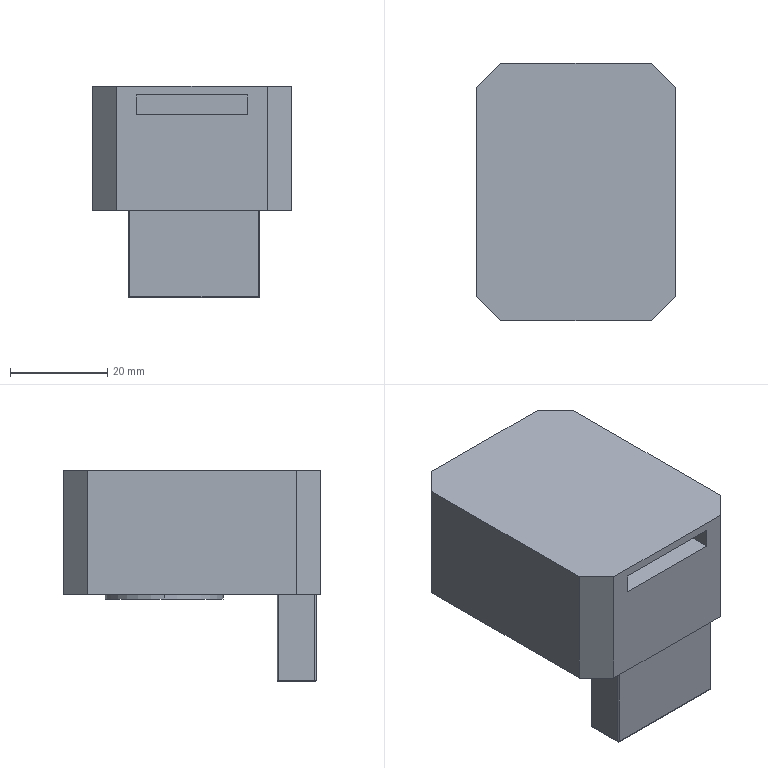Part | SolidWorks | features BaseBody 1 | 1 solid | 36 faces | box 41 x 53 x 43.5 mm | volume 58117 mm3 | plane 21 | cylinder 10 | spline 5 | commonest cylinder face diameters 0.5 x8 24.262 x2
STEP:
#1=CARTESIAN_POINT('',(6.903,-41.356,-17.75));
#2=VERTEX_POINT('',#1);
#3=CARTESIAN_POINT('',(6.977,-41.179,-17.75));
#4=VERTEX_POINT('',#3);
#5=CARTESIAN_POINT('',(6.727,-41.179,-17.75));
#6=DIRECTION('',(0.,0.,1.));
#7=DIRECTION('',(-1.,0.,0.));
#8=AXIS2_PLACEMENT_3D('',#5,#6,#7);
#9=CIRCLE('',#8,0.25);
#10=EDGE_CURVE('',#2,#4,#9,.T.);
#11=ORIENTED_EDGE('',*,*,#10,.F.);
#12=CARTESIAN_POINT('',(6.903,-41.179,-17.927));
#13=VERTEX_POINT('',#12);
#14=CARTESIAN_POINT('',(6.727,-41.179,-17.75));
#15=DIRECTION('',(0.5774,0.5774,0.5774));
#16=DIRECTION('',(-0.7071,0.,0.7071));
#17=AXIS2_PLACEMENT_3D('',#14,#15,#16);
#18=CIRCLE('',#17,0.25);
#19=EDGE_CURVE('',#2,#13,#18,.T.);
#20=ORIENTED_EDGE('',*,*,#19,.T.);
#21=CARTESIAN_POINT('',(6.727,-41.179,-17.75));
#22=DIRECTION('',(0.,1.,0.));
#23=DIRECTION('',(-1.,0.,0.));
#24=AXIS2_PLACEMENT_3D('',#21,#22,#23);
#25=CIRCLE('',#24,0.25);
#26=EDGE_CURVE('',#4,#13,#25,.T.);
#27=ORIENTED_EDGE('',*,*,#26,.F.);
#28=EDGE_LOOP('',(#11,#20,#27));
#29=FACE_OUTER_BOUND('',#28,.T.);
#30=CARTESIAN_POINT('',(6.903,-41.357,-17.749));
#31=CARTESIAN_POINT('',(6.944,-41.315,-17.707));
#32=CARTESIAN_POINT('',(6.968,-41.251,-17.684));
#33=CARTESIAN_POINT('',(6.968,-41.179,-17.684));
#34=CARTESIAN_POINT('',(6.941,-41.32,-17.824));
#35=CARTESIAN_POINT('',(6.974,-41.287,-17.791));
#36=CARTESIAN_POINT('',(6.992,-41.236,-17.773));
#37=CARTESIAN_POINT('',(6.992,-41.179,-17.773));
#38=CARTESIAN_POINT('',(6.941,-41.255,-17.889));
#39=CARTESIAN_POINT('',(6.959,-41.237,-17.872));
#40=CARTESIAN_POINT('',(6.969,-41.21,-17.862));
#41=CARTESIAN_POINT('',(6.969,-41.179,-17.862));
#42=CARTESIAN_POINT('',(6.903,-41.179,-17.927));
#43=CARTESIAN_POINT('',(6.903,-41.179,-17.927));
#44=CARTESIAN_POINT('',(6.903,-41.179,-17.927));
#45=CARTESIAN_POINT('',(6.903,-41.179,-17.927));
#46=(BOUNDED_SURFACE()B_SPLINE_SURFACE(3,3,((#30,#31,#32,#33),(#34,#35,#36,#37),(#38,#39,#40,#41),(#42,#43,#44,#45)),.UNSPECIFIED.,.F.,.F.,.F.)B_SPLINE_SURFACE_WITH_KNOTS((4,4),(4,4),(0.,1.),(0.,1.),.UNSPECIFIED.)GEOMETRIC_REPRESENTATION_ITEM()RATIONAL_B_SPLINE_SURFACE(((1.,0.9254,0.9254,1.),(0.9096,0.8418,0.8418,0.9096),(0.9096,0.8418,0.8418,0.9096),(1.,0.9254,0.9254,1.)))REPRESENTATION_ITEM('')SURFACE());
#47=ADVANCED_FACE('',(#29),#46,.T.);
#48=CARTESIAN_POINT('',(-19.304,-10.179,0.));
#49=VERTEX_POINT('',#48);
#50=CARTESIAN_POINT('',(4.957,-10.179,0.));
#51=VERTEX_POINT('',#50);
#52=CARTESIAN_POINT('',(-7.173,-10.179,0.));
#53=DIRECTION('',(0.,0.,-1.));
#54=DIRECTION('',(-1.,0.,0.));
#55=AXIS2_PLACEMENT_3D('',#52,#53,#54);
#56=CIRCLE('',#55,12.131);
#57=EDGE_CURVE('',#49,#51,#56,.T.);
#58=ORIENTED_EDGE('',*,*,#57,.T.);
#59=CARTESIAN_POINT('',(4.957,-10.179,-1.));
#60=VERTEX_POINT('',#59);
#61=CARTESIAN_POINT('',(4.957,-10.179,0.));
#62=DIRECTION('',(0.,0.,-1.));
#63=VECTOR('',#62,1000.);
#64=LINE('',#61,#63);
#65=EDGE_CURVE('',#51,#60,#64,.T.);
#66=ORIENTED_EDGE('',*,*,#65,.T.);
#67=CARTESIAN_POINT('',(-19.304,-10.179,-1.));
#68=VERTEX_POINT('',#67);
#69=CARTESIAN_POINT('',(-7.173,-10.179,-1.));
#70=DIRECTION('',(0.,0.,1.));
#71=DIRECTION('',(-1.,0.,0.));
#72=AXIS2_PLACEMENT_3D('',#69,#70,#71);
#73=CIRCLE('',#72,12.131);
#74=EDGE_CURVE('',#60,#68,#73,.T.);
#75=ORIENTED_EDGE('',*,*,#74,.T.);
#76=CARTESIAN_POINT('',(-19.304,-10.179,0.));
#77=DIRECTION('',(0.,0.,-1.));
#78=VECTOR('',#77,1000.);
#79=LINE('',#76,#78);
#80=EDGE_CURVE('',#49,#68,#79,.T.);
#81=ORIENTED_EDGE('',*,*,#80,.F.);
#82=EDGE_LOOP('',(#58,#66,#75,#81));
#83=FACE_OUTER_BOUND('',#82,.T.);
#84=CARTESIAN_POINT('',(-7.173,-10.179,0.));
#85=DIRECTION('',(0.,0.,-1.));
#86=DIRECTION('',(-1.,0.,0.));
#87=AXIS2_PLACEMENT_3D('',#84,#85,#86);
#88=CYLINDRICAL_SURFACE('',#87,12.131);
#89=ADVANCED_FACE('',(#83),#88,.T.);
#90=CARTESIAN_POINT('',(-22.423,10.571,25.5));
#91=VERTEX_POINT('',#90);
#92=CARTESIAN_POINT('',(-27.423,5.571,25.5));
#93=VERTEX_POINT('',#92);
#94=CARTESIAN_POINT('',(-22.423,10.571,25.5));
#95=DIRECTION('',(-0.7071,-0.7071,0.));
#96=VECTOR('',#95,1000.);
#97=LINE('',#94,#96);
#98=EDGE_CURVE('',#91,#93,#97,.T.);
#99=ORIENTED_EDGE('',*,*,#98,.T.);
#100=CARTESIAN_POINT('',(-27.423,-37.429,25.5));
#101=VERTEX_POINT('',#100);
#102=CARTESIAN_POINT('',(-27.423,-15.929,25.5));
#103=DIRECTION('',(0.,-1.,0.));
#104=VECTOR('',#103,1000.);
#105=LINE('',#102,#104);
#106=EDGE_CURVE('',#93,#101,#105,.T.);
#107=ORIENTED_EDGE('',*,*,#106,.T.);
#108=CARTESIAN_POINT('',(-22.423,-42.429,25.5));
#109=VERTEX_POINT('',#108);
#110=CARTESIAN_POINT('',(-27.423,-37.429,25.5));
#111=DIRECTION('',(0.7071,-0.7071,0.));
#112=VECTOR('',#111,1000.);
#113=LINE('',#110,#112);
#114=EDGE_CURVE('',#101,#109,#113,.T.);
#115=ORIENTED_EDGE('',*,*,#114,.T.);
#116=CARTESIAN_POINT('',(8.577,-42.429,25.5));
#117=VERTEX_POINT('',#116);
#118=CARTESIAN_POINT('',(-6.923,-42.429,25.5));
#119=DIRECTION('',(1.,0.,0.));
#120=VECTOR('',#119,1000.);
#121=LINE('',#118,#120);
#122=EDGE_CURVE('',#109,#117,#121,.T.);
#123=ORIENTED_EDGE('',*,*,#122,.T.);
#124=CARTESIAN_POINT('',(13.577,-37.429,25.5));
#125=VERTEX_POINT('',#124);
#126=CARTESIAN_POINT('',(8.577,-42.429,25.5));
#127=DIRECTION('',(0.7071,0.7071,0.));
#128=VECTOR('',#127,1000.);
#129=LINE('',#126,#128);
#130=EDGE_CURVE('',#117,#125,#129,.T.);
#131=ORIENTED_EDGE('',*,*,#130,.T.);
#132=CARTESIAN_POINT('',(13.577,5.571,25.5));
#133=VERTEX_POINT('',#132);
#134=CARTESIAN_POINT('',(13.577,-15.929,25.5));
#135=DIRECTION('',(0.,1.,0.));
#136=VECTOR('',#135,1000.);
#137=LINE('',#134,#136);
#138=EDGE_CURVE('',#125,#133,#137,.T.);
#139=ORIENTED_EDGE('',*,*,#138,.T.);
#140=CARTESIAN_POINT('',(8.577,10.571,25.5));
#141=VERTEX_POINT('',#140);
#142=CARTESIAN_POINT('',(13.577,5.571,25.5));
#143=DIRECTION('',(-0.7071,0.7071,0.));
#144=VECTOR('',#143,1000.);
#145=LINE('',#142,#144);
#146=EDGE_CURVE('',#133,#141,#145,.T.);
#147=ORIENTED_EDGE('',*,*,#146,.T.);
#148=CARTESIAN_POINT('',(-6.923,10.571,25.5));
#149=DIRECTION('',(-1.,0.,0.));
#150=VECTOR('',#149,1000.);
#151=LINE('',#148,#150);
#152=EDGE_CURVE('',#141,#91,#151,.T.);
#153=ORIENTED_EDGE('',*,*,#152,.T.);
#154=EDGE_LOOP('',(#99,#107,#115,#123,#131,#139,#147,#153));
#155=FACE_OUTER_BOUND('',#154,.T.);
#156=CARTESIAN_POINT('',(-6.923,-15.929,25.5));
#157=DIRECTION('',(0.,0.,1.));
#158=DIRECTION('',(1.,0.,0.));
#159=AXIS2_PLACEMENT_3D('',#156,#157,#158);
#160=PLANE('',#159);
#161=ADVANCED_FACE('',(#155),#160,.T.);
#162=CARTESIAN_POINT('',(-27.423,5.571,0.));
#163=VERTEX_POINT('',#162);
#164=CARTESIAN_POINT('',(-27.423,5.571,0.));
#165=DIRECTION('',(0.,0.,-1.));
#166=VECTOR('',#165,1000.);
#167=LINE('',#164,#166);
#168=EDGE_CURVE('',#93,#163,#167,.T.);
#169=ORIENTED_EDGE('',*,*,#168,.T.);
#170=CARTESIAN_POINT('',(-27.423,-37.429,0.));
#171=VERTEX_POINT('',#170);
#172=CARTESIAN_POINT('',(-27.423,-42.429,0.));
#173=DIRECTION('',(0.,-1.,0.));
#174=VECTOR('',#173,1000.);
#175=LINE('',#172,#174);
#176=EDGE_CURVE('',#163,#171,#175,.T.);
#177=ORIENTED_EDGE('',*,*,#176,.T.);
#178=CARTESIAN_POINT('',(-27.423,-37.429,0.));
#179=DIRECTION('',(0.,0.,1.));
#180=VECTOR('',#179,1000.);
#181=LINE('',#178,#180);
#182=EDGE_CURVE('',#171,#101,#181,.T.);
#183=ORIENTED_EDGE('',*,*,#182,.T.);
#184=ORIENTED_EDGE('',*,*,#106,.F.);
#185=EDGE_LOOP('',(#169,#177,#183,#184));
#186=FACE_OUTER_BOUND('',#185,.T.);
#187=CARTESIAN_POINT('',(-27.423,-42.429,0.));
#188=DIRECTION('',(-1.,0.,0.));
#189=DIRECTION('',(0.,0.,1.));
#190=AXIS2_PLACEMENT_3D('',#187,#188,#189);
#191=PLANE('',#190);
#192=ADVANCED_FACE('',(#186),#191,.T.);
#193=CARTESIAN_POINT('',(-22.423,10.571,0.));
#194=VERTEX_POINT('',#193);
#195=CARTESIAN_POINT('',(-24.923,8.071,0.));
#196=DIRECTION('',(-0.7071,-0.7071,0.));
#197=VECTOR('',#196,1000.);
#198=LINE('',#195,#197);
#199=EDGE_CURVE('',#194,#163,#198,.T.);
#200=ORIENTED_EDGE('',*,*,#199,.T.);
#201=ORIENTED_EDGE('',*,*,#168,.F.);
#202=ORIENTED_EDGE('',*,*,#98,.F.);
#203=CARTESIAN_POINT('',(-22.423,10.571,0.));
#204=DIRECTION('',(0.,0.,-1.));
#205=VECTOR('',#204,1000.);
#206=LINE('',#203,#205);
#207=EDGE_CURVE('',#91,#194,#206,.T.);
#208=ORIENTED_EDGE('',*,*,#207,.T.);
#209=EDGE_LOOP('',(#200,#201,#202,#208));
#210=FACE_OUTER_BOUND('',#209,.T.);
#211=CARTESIAN_POINT('',(-24.923,8.071,0.));
#212=DIRECTION('',(-0.7071,0.7071,0.));
#213=DIRECTION('',(-0.7071,-0.7071,0.));
#214=AXIS2_PLACEMENT_3D('',#211,#212,#213);
#215=PLANE('',#214);
#216=ADVANCED_FACE('',(#210),#215,.T.);
#217=ORIENTED_EDGE('',*,*,#207,.F.);
#218=ORIENTED_EDGE('',*,*,#152,.F.);
#219=CARTESIAN_POINT('',(8.577,10.571,0.));
#220=VERTEX_POINT('',#219);
#221=CARTESIAN_POINT('',(8.577,10.571,0.));
#222=DIRECTION('',(0.,0.,-1.));
#223=VECTOR('',#222,1000.);
#224=LINE('',#221,#223);
#225=EDGE_CURVE('',#141,#220,#224,.T.);
#226=ORIENTED_EDGE('',*,*,#225,.T.);
#227=CARTESIAN_POINT('',(-27.423,10.571,0.));
#228=DIRECTION('',(-1.,0.,0.));
#229=VECTOR('',#228,1000.);
#230=LINE('',#227,#229);
#231=EDGE_CURVE('',#220,#194,#230,.T.);
#232=ORIENTED_EDGE('',*,*,#231,.T.);
#233=EDGE_LOOP('',(#217,#218,#226,#232));
#234=FACE_OUTER_BOUND('',#233,.T.);
#235=CARTESIAN_POINT('',(-27.423,10.571,0.));
#236=DIRECTION('',(0.,1.,0.));
#237=DIRECTION('',(0.,0.,1.));
#238=AXIS2_PLACEMENT_3D('',#235,#236,#237);
#239=PLANE('',#238);
#240=ADVANCED_FACE('',(#234),#239,.T.);
#241=CARTESIAN_POINT('',(13.577,5.571,0.));
#242=VERTEX_POINT('',#241);
#243=CARTESIAN_POINT('',(11.077,8.071,0.));
#244=DIRECTION('',(-0.7071,0.7071,0.));
#245=VECTOR('',#244,1000.);
#246=LINE('',#243,#245);
#247=EDGE_CURVE('',#242,#220,#246,.T.);
#248=ORIENTED_EDGE('',*,*,#247,.T.);
#249=ORIENTED_EDGE('',*,*,#225,.F.);
#250=ORIENTED_EDGE('',*,*,#146,.F.);
#251=CARTESIAN_POINT('',(13.577,5.571,0.));
#252=DIRECTION('',(0.,0.,-1.));
#253=VECTOR('',#252,1000.);
#254=LINE('',#251,#253);
#255=EDGE_CURVE('',#133,#242,#254,.T.);
#256=ORIENTED_EDGE('',*,*,#255,.T.);
#257=EDGE_LOOP('',(#248,#249,#250,#256));
#258=FACE_OUTER_BOUND('',#257,.T.);
#259=CARTESIAN_POINT('',(11.077,8.071,0.));
#260=DIRECTION('',(0.7071,0.7071,0.));
#261=DIRECTION('',(-0.7071,0.7071,0.));
#262=AXIS2_PLACEMENT_3D('',#259,#260,#261);
#263=PLANE('',#262);
#264=ADVANCED_FACE('',(#258),#263,.T.);
#265=ORIENTED_EDGE('',*,*,#255,.F.);
#266=ORIENTED_EDGE('',*,*,#138,.F.);
#267=CARTESIAN_POINT('',(13.577,-37.429,0.));
#268=VERTEX_POINT('',#267);
#269=CARTESIAN_POINT('',(13.577,-37.429,0.));
#270=DIRECTION('',(0.,0.,-1.));
#271=VECTOR('',#270,1000.);
#272=LINE('',#269,#271);
#273=EDGE_CURVE('',#125,#268,#272,.T.);
#274=ORIENTED_EDGE('',*,*,#273,.T.);
#275=CARTESIAN_POINT('',(13.577,10.571,0.));
#276=DIRECTION('',(0.,1.,0.));
#277=VECTOR('',#276,1000.);
#278=LINE('',#275,#277);
#279=EDGE_CURVE('',#268,#242,#278,.T.);
#280=ORIENTED_EDGE('',*,*,#279,.T.);
#281=EDGE_LOOP('',(#265,#266,#274,#280));
#282=FACE_OUTER_BOUND('',#281,.T.);
#283=CARTESIAN_POINT('',(13.577,10.571,0.));
#284=DIRECTION('',(1.,0.,0.));
#285=DIRECTION('',(0.,0.,-1.));
#286=AXIS2_PLACEMENT_3D('',#283,#284,#285);
#287=PLANE('',#286);
#288=ADVANCED_FACE('',(#282),#287,.T.);
#289=CARTESIAN_POINT('',(8.577,-42.429,0.));
#290=VERTEX_POINT('',#289);
#291=CARTESIAN_POINT('',(11.077,-39.929,0.));
#292=DIRECTION('',(0.7071,0.7071,0.));
#293=VECTOR('',#292,1000.);
#294=LINE('',#291,#293);
#295=EDGE_CURVE('',#290,#268,#294,.T.);
#296=ORIENTED_EDGE('',*,*,#295,.T.);
#297=ORIENTED_EDGE('',*,*,#273,.F.);
#298=ORIENTED_EDGE('',*,*,#130,.F.);
#299=CARTESIAN_POINT('',(8.577,-42.429,0.));
#300=DIRECTION('',(0.,0.,-1.));
#301=VECTOR('',#300,1000.);
#302=LINE('',#299,#301);
#303=EDGE_CURVE('',#117,#290,#302,.T.);
#304=ORIENTED_EDGE('',*,*,#303,.T.);
#305=EDGE_LOOP('',(#296,#297,#298,#304));
#306=FACE_OUTER_BOUND('',#305,.T.);
#307=CARTESIAN_POINT('',(11.077,-39.929,0.));
#308=DIRECTION('',(0.7071,-0.7071,0.));
#309=DIRECTION('',(0.7071,0.7071,0.));
#310=AXIS2_PLACEMENT_3D('',#307,#308,#309);
#311=PLANE('',#310);
#312=ADVANCED_FACE('',(#306),#311,.T.);
#313=CARTESIAN_POINT('',(-18.423,-42.429,19.7));
#314=VERTEX_POINT('',#313);
#315=CARTESIAN_POINT('',(-18.423,-42.429,23.7));
#316=VERTEX_POINT('',#315);
#317=CARTESIAN_POINT('',(-18.423,-42.429,0.));
#318=DIRECTION('',(0.,0.,1.));
#319=VECTOR('',#318,1000.);
#320=LINE('',#317,#319);
#321=EDGE_CURVE('',#314,#316,#320,.T.);
#322=ORIENTED_EDGE('',*,*,#321,.T.);
#323=CARTESIAN_POINT('',(4.577,-42.429,23.7));
#324=VERTEX_POINT('',#323);
#325=CARTESIAN_POINT('',(13.577,-42.429,23.7));
#326=DIRECTION('',(1.,0.,0.));
#327=VECTOR('',#326,1000.);
#328=LINE('',#325,#327);
#329=EDGE_CURVE('',#316,#324,#328,.T.);
#330=ORIENTED_EDGE('',*,*,#329,.T.);
#331=CARTESIAN_POINT('',(4.577,-42.429,19.7));
#332=VERTEX_POINT('',#331);
#333=CARTESIAN_POINT('',(4.577,-42.429,0.));
#334=DIRECTION('',(0.,0.,-1.));
#335=VECTOR('',#334,1000.);
#336=LINE('',#333,#335);
#337=EDGE_CURVE('',#324,#332,#336,.T.);
#338=ORIENTED_EDGE('',*,*,#337,.T.);
#339=CARTESIAN_POINT('',(13.577,-42.429,19.7));
#340=DIRECTION('',(-1.,0.,0.));
#341=VECTOR('',#340,1000.);
#342=LINE('',#339,#341);
#343=EDGE_CURVE('',#332,#314,#342,.T.);
#344=ORIENTED_EDGE('',*,*,#343,.T.);
#345=EDGE_LOOP('',(#322,#330,#338,#344));
#346=FACE_BOUND('',#345,.T.);
#347=ORIENTED_EDGE('',*,*,#303,.F.);
#348=ORIENTED_EDGE('',*,*,#122,.F.);
#349=CARTESIAN_POINT('',(-22.423,-42.429,0.));
#350=VERTEX_POINT('',#349);
#351=CARTESIAN_POINT('',(-22.423,-42.429,0.));
#352=DIRECTION('',(0.,0.,-1.));
#353=VECTOR('',#352,1000.);
#354=LINE('',#351,#353);
#355=EDGE_CURVE('',#109,#350,#354,.T.);
#356=ORIENTED_EDGE('',*,*,#355,.T.);
#357=CARTESIAN_POINT('',(13.577,-42.429,0.));
#358=DIRECTION('',(1.,0.,0.));
#359=VECTOR('',#358,1000.);
#360=LINE('',#357,#359);
#361=EDGE_CURVE('',#350,#290,#360,.T.);
#362=ORIENTED_EDGE('',*,*,#361,.T.);
#363=EDGE_LOOP('',(#347,#348,#356,#362));
#364=FACE_OUTER_BOUND('',#363,.T.);
#365=CARTESIAN_POINT('',(13.577,-42.429,0.));
#366=DIRECTION('',(0.,-1.,0.));
#367=DIRECTION('',(0.,0.,-1.));
#368=AXIS2_PLACEMENT_3D('',#365,#366,#367);
#369=PLANE('',#368);
#370=ADVANCED_FACE('',(#346,#364),#369,.T.);
#371=CARTESIAN_POINT('',(-24.923,-39.929,0.));
#372=DIRECTION('',(0.7071,-0.7071,0.));
#373=VECTOR('',#372,1000.);
#374=LINE('',#371,#373);
#375=EDGE_CURVE('',#171,#350,#374,.T.);
#376=ORIENTED_EDGE('',*,*,#375,.T.);
#377=ORIENTED_EDGE('',*,*,#355,.F.);
#378=ORIENTED_EDGE('',*,*,#114,.F.);
#379=ORIENTED_EDGE('',*,*,#182,.F.);
#380=EDGE_LOOP('',(#376,#377,#378,#379));
#381=FACE_OUTER_BOUND('',#380,.T.);
#382=CARTESIAN_POINT('',(-24.923,-39.929,0.));
#383=DIRECTION('',(-0.7071,-0.7071,0.));
#384=DIRECTION('',(0.7071,-0.7071,0.));
#385=AXIS2_PLACEMENT_3D('',#382,#383,#384);
#386=PLANE('',#385);
#387=ADVANCED_FACE('',(#381),#386,.T.);
#388=CARTESIAN_POINT('',(-19.773,-41.429,0.));
#389=VERTEX_POINT('',#388);
#390=CARTESIAN_POINT('',(-20.023,-41.179,0.));
#391=VERTEX_POINT('',#390);
#392=CARTESIAN_POINT('',(-19.773,-41.179,0.));
#393=DIRECTION('',(0.,0.,-1.));
#394=DIRECTION('',(-1.,0.,0.));
#395=AXIS2_PLACEMENT_3D('',#392,#393,#394);
#396=CIRCLE('',#395,0.25);
#397=EDGE_CURVE('',#389,#391,#396,.T.);
#398=ORIENTED_EDGE('',*,*,#397,.F.);
#399=CARTESIAN_POINT('',(6.727,-41.429,0.));
#400=VERTEX_POINT('',#399);
#401=CARTESIAN_POINT('',(-6.923,-41.429,0.));
#402=DIRECTION('',(-1.,0.,0.));
#403=VECTOR('',#402,1000.);
#404=LINE('',#401,#403);
#405=EDGE_CURVE('',#400,#389,#404,.T.);
#406=ORIENTED_EDGE('',*,*,#405,.F.);
#407=CARTESIAN_POINT('',(6.977,-41.179,0.));
#408=VERTEX_POINT('',#407);
#409=CARTESIAN_POINT('',(6.727,-41.179,0.));
#410=DIRECTION('',(0.,0.,-1.));
#411=DIRECTION('',(-1.,0.,0.));
#412=AXIS2_PLACEMENT_3D('',#409,#410,#411);
#413=CIRCLE('',#412,0.25);
#414=EDGE_CURVE('',#408,#400,#413,.T.);
#415=ORIENTED_EDGE('',*,*,#414,.F.);
#416=CARTESIAN_POINT('',(6.977,-33.679,0.));
#417=VERTEX_POINT('',#416);
#418=CARTESIAN_POINT('',(6.977,-15.929,0.));
#419=DIRECTION('',(0.,-1.,0.));
#420=VECTOR('',#419,1000.);
#421=LINE('',#418,#420);
#422=EDGE_CURVE('',#417,#408,#421,.T.);
#423=ORIENTED_EDGE('',*,*,#422,.F.);
#424=CARTESIAN_POINT('',(6.727,-33.429,0.));
#425=VERTEX_POINT('',#424);
#426=CARTESIAN_POINT('',(6.727,-33.679,0.));
#427=DIRECTION('',(0.,0.,-1.));
#428=DIRECTION('',(-1.,0.,0.));
#429=AXIS2_PLACEMENT_3D('',#426,#427,#428);
#430=CIRCLE('',#429,0.25);
#431=EDGE_CURVE('',#425,#417,#430,.T.);
#432=ORIENTED_EDGE('',*,*,#431,.F.);
#433=CARTESIAN_POINT('',(-19.773,-33.429,0.));
#434=VERTEX_POINT('',#433);
#435=CARTESIAN_POINT('',(-6.923,-33.429,0.));
#436=DIRECTION('',(1.,0.,0.));
#437=VECTOR('',#436,1000.);
#438=LINE('',#435,#437);
#439=EDGE_CURVE('',#434,#425,#438,.T.);
#440=ORIENTED_EDGE('',*,*,#439,.F.);
#441=CARTESIAN_POINT('',(-20.023,-33.679,0.));
#442=VERTEX_POINT('',#441);
#443=CARTESIAN_POINT('',(-19.773,-33.679,0.));
#444=DIRECTION('',(0.,0.,-1.));
#445=DIRECTION('',(-1.,0.,0.));
#446=AXIS2_PLACEMENT_3D('',#443,#444,#445);
#447=CIRCLE('',#446,0.25);
#448=EDGE_CURVE('',#442,#434,#447,.T.);
#449=ORIENTED_EDGE('',*,*,#448,.F.);
#450=CARTESIAN_POINT('',(-20.023,-15.929,0.));
#451=DIRECTION('',(0.,1.,0.));
#452=VECTOR('',#451,1000.);
#453=LINE('',#450,#452);
#454=EDGE_CURVE('',#391,#442,#453,.T.);
#455=ORIENTED_EDGE('',*,*,#454,.F.);
#456=EDGE_LOOP('',(#398,#406,#415,#423,#432,#440,#449,#455));
#457=FACE_BOUND('',#456,.T.);
#458=ORIENTED_EDGE('',*,*,#57,.F.);
#459=CARTESIAN_POINT('',(-7.173,-10.179,0.));
#460=DIRECTION('',(0.,0.,-1.));
#461=DIRECTION('',(-1.,0.,0.));
#462=AXIS2_PLACEMENT_3D('',#459,#460,#461);
#463=CIRCLE('',#462,12.131);
#464=EDGE_CURVE('',#51,#49,#463,.T.);
#465=ORIENTED_EDGE('',*,*,#464,.F.);
#466=EDGE_LOOP('',(#458,#465));
#467=FACE_BOUND('',#466,.T.);
#468=ORIENTED_EDGE('',*,*,#176,.F.);
#469=ORIENTED_EDGE('',*,*,#199,.F.);
#470=ORIENTED_EDGE('',*,*,#231,.F.);
#471=ORIENTED_EDGE('',*,*,#247,.F.);
#472=ORIENTED_EDGE('',*,*,#279,.F.);
#473=ORIENTED_EDGE('',*,*,#295,.F.);
#474=ORIENTED_EDGE('',*,*,#361,.F.);
#475=ORIENTED_EDGE('',*,*,#375,.F.);
#476=EDGE_LOOP('',(#468,#469,#470,#471,#472,#473,#474,#475));
#477=FACE_OUTER_BOUND('',#476,.T.);
#478=CARTESIAN_POINT('',(-6.923,-15.929,0.));
#479=DIRECTION('',(0.,0.,1.));
#480=DIRECTION('',(1.,0.,0.));
#481=AXIS2_PLACEMENT_3D('',#478,#479,#480);
#482=PLANE('',#481);
#483=ADVANCED_FACE('',(#457,#467,#477),#482,.F.);
#484=CARTESIAN_POINT('',(4.577,-38.429,23.7));
#485=VERTEX_POINT('',#484);
#486=CARTESIAN_POINT('',(4.577,-42.429,23.7));
#487=DIRECTION('',(0.,1.,0.));
#488=VECTOR('',#487,1000.);
#489=LINE('',#486,#488);
#490=EDGE_CURVE('',#324,#485,#489,.T.);
#491=ORIENTED_EDGE('',*,*,#490,.F.);
#492=ORIENTED_EDGE('',*,*,#329,.F.);
#493=CARTESIAN_POINT('',(-18.423,-38.429,23.7));
#494=VERTEX_POINT('',#493);
#495=CARTESIAN_POINT('',(-18.423,-42.429,23.7));
#496=DIRECTION('',(0.,-1.,0.));
#497=VECTOR('',#496,1000.);
#498=LINE('',#495,#497);
#499=EDGE_CURVE('',#494,#316,#498,.T.);
#500=ORIENTED_EDGE('',*,*,#499,.F.);
#501=CARTESIAN_POINT('',(4.577,-38.429,23.7));
#502=DIRECTION('',(-1.,0.,0.));
#503=VECTOR('',#502,1000.);
#504=LINE('',#501,#503);
#505=EDGE_CURVE('',#485,#494,#504,.T.);
#506=ORIENTED_EDGE('',*,*,#505,.F.);
#507=EDGE_LOOP('',(#491,#492,#500,#506));
#508=FACE_OUTER_BOUND('',#507,.T.);
#509=CARTESIAN_POINT('',(4.577,-42.429,23.7));
#510=DIRECTION('',(0.,0.,1.));
#511=DIRECTION('',(1.,0.,0.));
#512=AXIS2_PLACEMENT_3D('',#509,#510,#511);
#513=PLANE('',#512);
#514=ADVANCED_FACE('',(#508),#513,.F.);
#515=ORIENTED_EDGE('',*,*,#499,.T.);
#516=ORIENTED_EDGE('',*,*,#321,.F.);
#517=CARTESIAN_POINT('',(-18.423,-38.429,19.7));
#518=VERTEX_POINT('',#517);
#519=CARTESIAN_POINT('',(-18.423,-42.429,19.7));
#520=DIRECTION('',(0.,-1.,0.));
#521=VECTOR('',#520,1000.);
#522=LINE('',#519,#521);
#523=EDGE_CURVE('',#518,#314,#522,.T.);
#524=ORIENTED_EDGE('',*,*,#523,.F.);
#525=CARTESIAN_POINT('',(-18.423,-38.429,23.7));
#526=DIRECTION('',(0.,0.,-1.));
#527=VECTOR('',#526,1000.);
#528=LINE('',#525,#527);
#529=EDGE_CURVE('',#494,#518,#528,.T.);
#530=ORIENTED_EDGE('',*,*,#529,.F.);
#531=EDGE_LOOP('',(#515,#516,#524,#530));
#532=FACE_OUTER_BOUND('',#531,.T.);
#533=CARTESIAN_POINT('',(-18.423,-42.429,23.7));
#534=DIRECTION('',(-1.,0.,0.));
#535=DIRECTION('',(0.,0.,1.));
#536=AXIS2_PLACEMENT_3D('',#533,#534,#535);
#537=PLANE('',#536);
#538=ADVANCED_FACE('',(#532),#537,.F.);
#539=ORIENTED_EDGE('',*,*,#523,.T.);
#540=ORIENTED_EDGE('',*,*,#343,.F.);
#541=CARTESIAN_POINT('',(4.577,-38.429,19.7));
#542=VERTEX_POINT('',#541);
#543=CARTESIAN_POINT('',(4.577,-42.429,19.7));
#544=DIRECTION('',(0.,-1.,0.));
#545=VECTOR('',#544,1000.);
#546=LINE('',#543,#545);
#547=EDGE_CURVE('',#542,#332,#546,.T.);
#548=ORIENTED_EDGE('',*,*,#547,.F.);
#549=CARTESIAN_POINT('',(-18.423,-38.429,19.7));
#550=DIRECTION('',(1.,0.,0.));
#551=VECTOR('',#550,1000.);
#552=LINE('',#549,#551);
#553=EDGE_CURVE('',#518,#542,#552,.T.);
#554=ORIENTED_EDGE('',*,*,#553,.F.);
#555=EDGE_LOOP('',(#539,#540,#548,#554));
#556=FACE_OUTER_BOUND('',#555,.T.);
#557=CARTESIAN_POINT('',(-18.423,-42.429,19.7));
#558=DIRECTION('',(0.,0.,-1.));
#559=DIRECTION('',(-1.,0.,0.));
#560=AXIS2_PLACEMENT_3D('',#557,#558,#559);
#561=PLANE('',#560);
#562=ADVANCED_FACE('',(#556),#561,.F.);
#563=ORIENTED_EDGE('',*,*,#547,.T.);
#564=ORIENTED_EDGE('',*,*,#337,.F.);
#565=ORIENTED_EDGE('',*,*,#490,.T.);
#566=CARTESIAN_POINT('',(4.577,-38.429,19.7));
#567=DIRECTION('',(0.,0.,1.));
#568=VECTOR('',#567,1000.);
#569=LINE('',#566,#568);
#570=EDGE_CURVE('',#542,#485,#569,.T.);
#571=ORIENTED_EDGE('',*,*,#570,.F.);
#572=EDGE_LOOP('',(#563,#564,#565,#571));
#573=FACE_OUTER_BOUND('',#572,.T.);
#574=CARTESIAN_POINT('',(4.577,-42.429,19.7));
#575=DIRECTION('',(1.,0.,0.));
#576=DIRECTION('',(0.,0.,-1.));
#577=AXIS2_PLACEMENT_3D('',#574,#575,#576);
#578=PLANE('',#577);
#579=ADVANCED_FACE('',(#573),#578,.F.);
#580=CARTESIAN_POINT('',(-20.023,-41.179,-17.75));
#581=VERTEX_POINT('',#580);
#582=CARTESIAN_POINT('',(-20.023,-41.179,0.));
#583=DIRECTION('',(0.,0.,1.));
#584=VECTOR('',#583,1000.);
#585=LINE('',#582,#584);
#586=EDGE_CURVE('',#581,#391,#585,.T.);
#587=ORIENTED_EDGE('',*,*,#586,.T.);
#588=ORIENTED_EDGE('',*,*,#454,.T.);
#589=CARTESIAN_POINT('',(-20.023,-33.679,-17.75));
#590=VERTEX_POINT('',#589);
#591=CARTESIAN_POINT('',(-20.023,-33.679,0.));
#592=DIRECTION('',(0.,0.,-1.));
#593=VECTOR('',#592,1000.);
#594=LINE('',#591,#593);
#595=EDGE_CURVE('',#442,#590,#594,.T.);
#596=ORIENTED_EDGE('',*,*,#595,.T.);
#597=CARTESIAN_POINT('',(-20.023,-33.429,-17.75));
#598=DIRECTION('',(0.,-1.,0.));
#599=VECTOR('',#598,1000.);
#600=LINE('',#597,#599);
#601=EDGE_CURVE('',#590,#581,#600,.T.);
#602=ORIENTED_EDGE('',*,*,#601,.T.);
#603=EDGE_LOOP('',(#587,#588,#596,#602));
#604=FACE_OUTER_BOUND('',#603,.T.);
#605=CARTESIAN_POINT('',(-20.023,-33.429,0.));
#606=DIRECTION('',(-1.,0.,0.));
#607=DIRECTION('',(0.,0.,1.));
#608=AXIS2_PLACEMENT_3D('',#605,#606,#607);
#609=PLANE('',#608);
#610=ADVANCED_FACE('',(#604),#609,.T.);
#611=CARTESIAN_POINT('',(-19.773,-41.429,-17.75));
#612=VERTEX_POINT('',#611);
#613=CARTESIAN_POINT('',(-19.773,-41.429,0.));
#614=DIRECTION('',(0.,0.,-1.));
#615=VECTOR('',#614,1000.);
#616=LINE('',#613,#615);
#617=EDGE_CURVE('',#389,#612,#616,.T.);
#618=ORIENTED_EDGE('',*,*,#617,.T.);
#619=CARTESIAN_POINT('',(6.727,-41.429,-17.75));
#620=VERTEX_POINT('',#619);
#621=CARTESIAN_POINT('',(-20.023,-41.429,-17.75));
#622=DIRECTION('',(1.,0.,0.));
#623=VECTOR('',#622,1000.);
#624=LINE('',#621,#623);
#625=EDGE_CURVE('',#612,#620,#624,.T.);
#626=ORIENTED_EDGE('',*,*,#625,.T.);
#627=CARTESIAN_POINT('',(6.727,-41.429,0.));
#628=DIRECTION('',(0.,0.,1.));
#629=VECTOR('',#628,1000.);
#630=LINE('',#627,#629);
#631=EDGE_CURVE('',#620,#400,#630,.T.);
#632=ORIENTED_EDGE('',*,*,#631,.T.);
#633=ORIENTED_EDGE('',*,*,#405,.T.);
#634=EDGE_LOOP('',(#618,#626,#632,#633));
#635=FACE_OUTER_BOUND('',#634,.T.);
#636=CARTESIAN_POINT('',(-20.023,-41.429,0.));
#637=DIRECTION('',(0.,-1.,0.));
#638=DIRECTION('',(0.,0.,-1.));
#639=AXIS2_PLACEMENT_3D('',#636,#637,#638);
#640=PLANE('',#639);
#641=ADVANCED_FACE('',(#635),#640,.T.);
#642=CARTESIAN_POINT('',(6.977,-41.179,0.));
#643=DIRECTION('',(0.,0.,-1.));
#644=VECTOR('',#643,1000.);
#645=LINE('',#642,#644);
#646=EDGE_CURVE('',#408,#4,#645,.T.);
#647=ORIENTED_EDGE('',*,*,#646,.T.);
#648=CARTESIAN_POINT('',(6.977,-33.679,-17.75));
#649=VERTEX_POINT('',#648);
#650=CARTESIAN_POINT('',(6.977,-41.429,-17.75));
#651=DIRECTION('',(0.,1.,0.));
#652=VECTOR('',#651,1000.);
#653=LINE('',#650,#652);
#654=EDGE_CURVE('',#4,#649,#653,.T.);
#655=ORIENTED_EDGE('',*,*,#654,.T.);
#656=CARTESIAN_POINT('',(6.977,-33.679,0.));
#657=DIRECTION('',(0.,0.,1.));
#658=VECTOR('',#657,1000.);
#659=LINE('',#656,#658);
#660=EDGE_CURVE('',#649,#417,#659,.T.);
#661=ORIENTED_EDGE('',*,*,#660,.T.);
#662=ORIENTED_EDGE('',*,*,#422,.T.);
#663=EDGE_LOOP('',(#647,#655,#661,#662));
#664=FACE_OUTER_BOUND('',#663,.T.);
#665=CARTESIAN_POINT('',(6.977,-41.429,0.));
#666=DIRECTION('',(1.,0.,0.));
#667=DIRECTION('',(0.,0.,-1.));
#668=AXIS2_PLACEMENT_3D('',#665,#666,#667);
#669=PLANE('',#668);
#670=ADVANCED_FACE('',(#664),#669,.T.);
#671=CARTESIAN_POINT('',(-19.773,-33.429,-17.75));
#672=VERTEX_POINT('',#671);
#673=CARTESIAN_POINT('',(-19.773,-33.429,0.));
#674=DIRECTION('',(0.,0.,1.));
#675=VECTOR('',#674,1000.);
#676=LINE('',#673,#675);
#677=EDGE_CURVE('',#672,#434,#676,.T.);
#678=ORIENTED_EDGE('',*,*,#677,.T.);
#679=ORIENTED_EDGE('',*,*,#439,.T.);
#680=CARTESIAN_POINT('',(6.727,-33.429,-17.75));
#681=VERTEX_POINT('',#680);
#682=CARTESIAN_POINT('',(6.727,-33.429,0.));
#683=DIRECTION('',(0.,0.,-1.));
#684=VECTOR('',#683,1000.);
#685=LINE('',#682,#684);
#686=EDGE_CURVE('',#425,#681,#685,.T.);
#687=ORIENTED_EDGE('',*,*,#686,.T.);
#688=CARTESIAN_POINT('',(6.977,-33.429,-17.75));
#689=DIRECTION('',(-1.,0.,0.));
#690=VECTOR('',#689,1000.);
#691=LINE('',#688,#690);
#692=EDGE_CURVE('',#681,#672,#691,.T.);
#693=ORIENTED_EDGE('',*,*,#692,.T.);
#694=EDGE_LOOP('',(#678,#679,#687,#693));
#695=FACE_OUTER_BOUND('',#694,.T.);
#696=CARTESIAN_POINT('',(6.977,-33.429,0.));
#697=DIRECTION('',(0.,1.,0.));
#698=DIRECTION('',(0.,0.,1.));
#699=AXIS2_PLACEMENT_3D('',#696,#697,#698);
#700=PLANE('',#699);
#701=ADVANCED_FACE('',(#695),#700,.T.);
#702=ORIENTED_EDGE('',*,*,#65,.F.);
#703=ORIENTED_EDGE('',*,*,#464,.T.);
#704=ORIENTED_EDGE('',*,*,#80,.T.);
#705=CARTESIAN_POINT('',(-7.173,-10.179,-1.));
#706=DIRECTION('',(0.,0.,1.));
#707=DIRECTION('',(-1.,0.,0.));
#708=AXIS2_PLACEMENT_3D('',#705,#706,#707);
#709=CIRCLE('',#708,12.131);
#710=EDGE_CURVE('',#68,#60,#709,.T.);
#711=ORIENTED_EDGE('',*,*,#710,.T.);
#712=EDGE_LOOP('',(#702,#703,#704,#711));
#713=FACE_OUTER_BOUND('',#712,.T.);
#714=CARTESIAN_POINT('',(-7.173,-10.179,0.));
#715=DIRECTION('',(0.,0.,-1.));
#716=DIRECTION('',(-1.,0.,0.));
#717=AXIS2_PLACEMENT_3D('',#714,#715,#716);
#718=CYLINDRICAL_SURFACE('',#717,12.131);
#719=ADVANCED_FACE('',(#713),#718,.T.);
#720=ORIENTED_EDGE('',*,*,#505,.T.);
#721=ORIENTED_EDGE('',*,*,#529,.T.);
#722=ORIENTED_EDGE('',*,*,#553,.T.);
#723=ORIENTED_EDGE('',*,*,#570,.T.);
#724=EDGE_LOOP('',(#720,#721,#722,#723));
#725=FACE_OUTER_BOUND('',#724,.T.);
#726=CARTESIAN_POINT('',(-6.923,-38.429,21.7));
#727=DIRECTION('',(0.,1.,0.));
#728=DIRECTION('',(0.,0.,1.));
#729=AXIS2_PLACEMENT_3D('',#726,#727,#728);
#730=PLANE('',#729);
#731=ADVANCED_FACE('',(#725),#730,.F.);
#732=CARTESIAN_POINT('',(-19.773,-41.179,-17.75));
#733=DIRECTION('',(0.,0.,1.));
#734=DIRECTION('',(-1.,0.,0.));
#735=AXIS2_PLACEMENT_3D('',#732,#733,#734);
#736=CIRCLE('',#735,0.25);
#737=EDGE_CURVE('',#581,#612,#736,.T.);
#738=ORIENTED_EDGE('',*,*,#737,.T.);
#739=ORIENTED_EDGE('',*,*,#617,.F.);
#740=ORIENTED_EDGE('',*,*,#397,.T.);
#741=ORIENTED_EDGE('',*,*,#586,.F.);
#742=EDGE_LOOP('',(#738,#739,#740,#741));
#743=FACE_OUTER_BOUND('',#742,.T.);
#744=CARTESIAN_POINT('',(-19.773,-41.179,0.));
#745=DIRECTION('',(0.,0.,-1.));
#746=DIRECTION('',(-1.,0.,0.));
#747=AXIS2_PLACEMENT_3D('',#744,#745,#746);
#748=CYLINDRICAL_SURFACE('',#747,0.25);
#749=ADVANCED_FACE('',(#743),#748,.T.);
#750=CARTESIAN_POINT('',(-19.773,-33.679,-18.));
#751=VERTEX_POINT('',#750);
#752=CARTESIAN_POINT('',(-19.773,-33.679,-17.75));
#753=DIRECTION('',(0.,-1.,0.));
#754=DIRECTION('',(0.,0.,-1.));
#755=AXIS2_PLACEMENT_3D('',#752,#753,#754);
#756=CIRCLE('',#755,0.25);
#757=EDGE_CURVE('',#590,#751,#756,.T.);
#758=ORIENTED_EDGE('',*,*,#757,.T.);
#759=CARTESIAN_POINT('',(-19.773,-41.179,-18.));
#760=VERTEX_POINT('',#759);
#761=CARTESIAN_POINT('',(-19.773,-35.429,-18.));
#762=DIRECTION('',(0.,-1.,0.));
#763=VECTOR('',#762,1000.);
#764=LINE('',#761,#763);
#765=EDGE_CURVE('',#751,#760,#764,.T.);
#766=ORIENTED_EDGE('',*,*,#765,.T.);
#767=CARTESIAN_POINT('',(-19.773,-41.179,-17.75));
#768=DIRECTION('',(0.,1.,0.));
#769=DIRECTION('',(0.,0.,-1.));
#770=AXIS2_PLACEMENT_3D('',#767,#768,#769);
#771=CIRCLE('',#770,0.25);
#772=EDGE_CURVE('',#760,#581,#771,.T.);
#773=ORIENTED_EDGE('',*,*,#772,.T.);
#774=ORIENTED_EDGE('',*,*,#601,.F.);
#775=EDGE_LOOP('',(#758,#766,#773,#774));
#776=FACE_OUTER_BOUND('',#775,.T.);
#777=CARTESIAN_POINT('',(-19.773,-35.429,-17.75));
#778=DIRECTION('',(0.,-1.,0.));
#779=DIRECTION('',(0.,0.,-1.));
#780=AXIS2_PLACEMENT_3D('',#777,#778,#779);
#781=CYLINDRICAL_SURFACE('',#780,0.25);
#782=ADVANCED_FACE('',(#776),#781,.T.);
#783=CARTESIAN_POINT('',(-19.773,-33.679,-17.75));
#784=DIRECTION('',(0.,0.,1.));
#785=DIRECTION('',(-1.,0.,0.));
#786=AXIS2_PLACEMENT_3D('',#783,#784,#785);
#787=CIRCLE('',#786,0.25);
#788=EDGE_CURVE('',#672,#590,#787,.T.);
#789=ORIENTED_EDGE('',*,*,#788,.T.);
#790=ORIENTED_EDGE('',*,*,#595,.F.);
#791=ORIENTED_EDGE('',*,*,#448,.T.);
#792=ORIENTED_EDGE('',*,*,#677,.F.);
#793=EDGE_LOOP('',(#789,#790,#791,#792));
#794=FACE_OUTER_BOUND('',#793,.T.);
#795=CARTESIAN_POINT('',(-19.773,-33.679,0.));
#796=DIRECTION('',(0.,0.,-1.));
#797=DIRECTION('',(-1.,0.,0.));
#798=AXIS2_PLACEMENT_3D('',#795,#796,#797);
#799=CYLINDRICAL_SURFACE('',#798,0.25);
#800=ADVANCED_FACE('',(#794),#799,.T.);
#801=CARTESIAN_POINT('',(-19.773,-41.179,-17.75));
#802=DIRECTION('',(1.,0.,0.));
#803=DIRECTION('',(0.,0.,-1.));
#804=AXIS2_PLACEMENT_3D('',#801,#802,#803);
#805=CIRCLE('',#804,0.25);
#806=EDGE_CURVE('',#612,#760,#805,.T.);
#807=ORIENTED_EDGE('',*,*,#806,.T.);
#808=CARTESIAN_POINT('',(6.727,-41.179,-18.));
#809=VERTEX_POINT('',#808);
#810=CARTESIAN_POINT('',(-13.273,-41.179,-18.));
#811=DIRECTION('',(1.,0.,0.));
#812=VECTOR('',#811,1000.);
#813=LINE('',#810,#812);
#814=EDGE_CURVE('',#760,#809,#813,.T.);
#815=ORIENTED_EDGE('',*,*,#814,.T.);
#816=CARTESIAN_POINT('',(6.727,-41.179,-17.75));
#817=DIRECTION('',(-1.,0.,0.));
#818=DIRECTION('',(0.,0.,-1.));
#819=AXIS2_PLACEMENT_3D('',#816,#817,#818);
#820=CIRCLE('',#819,0.25);
#821=EDGE_CURVE('',#809,#620,#820,.T.);
#822=ORIENTED_EDGE('',*,*,#821,.T.);
#823=ORIENTED_EDGE('',*,*,#625,.F.);
#824=EDGE_LOOP('',(#807,#815,#822,#823));
#825=FACE_OUTER_BOUND('',#824,.T.);
#826=CARTESIAN_POINT('',(-13.273,-41.179,-17.75));
#827=DIRECTION('',(1.,0.,0.));
#828=DIRECTION('',(0.,0.,-1.));
#829=AXIS2_PLACEMENT_3D('',#826,#827,#828);
#830=CYLINDRICAL_SURFACE('',#829,0.25);
#831=ADVANCED_FACE('',(#825),#830,.T.);
#832=CARTESIAN_POINT('',(6.727,-41.179,-17.75));
#833=DIRECTION('',(0.,0.,1.));
#834=DIRECTION('',(-1.,0.,0.));
#835=AXIS2_PLACEMENT_3D('',#832,#833,#834);
#836=CIRCLE('',#835,0.25);
#837=EDGE_CURVE('',#620,#2,#836,.T.);
#838=ORIENTED_EDGE('',*,*,#837,.T.);
#839=ORIENTED_EDGE('',*,*,#10,.T.);
#840=ORIENTED_EDGE('',*,*,#646,.F.);
#841=ORIENTED_EDGE('',*,*,#414,.T.);
#842=ORIENTED_EDGE('',*,*,#631,.F.);
#843=EDGE_LOOP('',(#838,#839,#840,#841,#842));
#844=FACE_OUTER_BOUND('',#843,.T.);
#845=CARTESIAN_POINT('',(6.727,-41.179,0.));
#846=DIRECTION('',(0.,0.,-1.));
#847=DIRECTION('',(-1.,0.,0.));
#848=AXIS2_PLACEMENT_3D('',#845,#846,#847);
#849=CYLINDRICAL_SURFACE('',#848,0.25);
#850=ADVANCED_FACE('',(#844),#849,.T.);
#851=CARTESIAN_POINT('',(6.727,-41.179,-17.75));
#852=DIRECTION('',(0.,1.,0.));
#853=DIRECTION('',(-1.,0.,0.));
#854=AXIS2_PLACEMENT_3D('',#851,#852,#853);
#855=CIRCLE('',#854,0.25);
#856=EDGE_CURVE('',#13,#809,#855,.T.);
#857=ORIENTED_EDGE('',*,*,#856,.T.);
#858=CARTESIAN_POINT('',(6.727,-33.679,-18.));
#859=VERTEX_POINT('',#858);
#860=CARTESIAN_POINT('',(6.727,-39.429,-18.));
#861=DIRECTION('',(0.,1.,0.));
#862=VECTOR('',#861,1000.);
#863=LINE('',#860,#862);
#864=EDGE_CURVE('',#809,#859,#863,.T.);
#865=ORIENTED_EDGE('',*,*,#864,.T.);
#866=CARTESIAN_POINT('',(6.903,-33.679,-17.927));
#867=VERTEX_POINT('',#866);
#868=CARTESIAN_POINT('',(6.727,-33.679,-17.75));
#869=DIRECTION('',(0.,-1.,0.));
#870=DIRECTION('',(-1.,0.,0.));
#871=AXIS2_PLACEMENT_3D('',#868,#869,#870);
#872=CIRCLE('',#871,0.25);
#873=EDGE_CURVE('',#859,#867,#872,.T.);
#874=ORIENTED_EDGE('',*,*,#873,.T.);
#875=CARTESIAN_POINT('',(6.727,-33.679,-17.75));
#876=DIRECTION('',(0.,-1.,0.));
#877=DIRECTION('',(-1.,0.,0.));
#878=AXIS2_PLACEMENT_3D('',#875,#876,#877);
#879=CIRCLE('',#878,0.25);
#880=EDGE_CURVE('',#867,#649,#879,.T.);
#881=ORIENTED_EDGE('',*,*,#880,.T.);
#882=ORIENTED_EDGE('',*,*,#654,.F.);
#883=ORIENTED_EDGE('',*,*,#26,.T.);
#884=EDGE_LOOP('',(#857,#865,#874,#881,#882,#883));
#885=FACE_OUTER_BOUND('',#884,.T.);
#886=CARTESIAN_POINT('',(6.727,-39.429,-17.75));
#887=DIRECTION('',(0.,1.,0.));
#888=DIRECTION('',(-1.,0.,0.));
#889=AXIS2_PLACEMENT_3D('',#886,#887,#888);
#890=CYLINDRICAL_SURFACE('',#889,0.25);
#891=ADVANCED_FACE('',(#885),#890,.T.);
#892=CARTESIAN_POINT('',(6.727,-33.679,-17.75));
#893=DIRECTION('',(0.,0.,1.));
#894=DIRECTION('',(-1.,0.,0.));
#895=AXIS2_PLACEMENT_3D('',#892,#893,#894);
#896=CIRCLE('',#895,0.25);
#897=EDGE_CURVE('',#649,#681,#896,.T.);
#898=ORIENTED_EDGE('',*,*,#897,.T.);
#899=ORIENTED_EDGE('',*,*,#686,.F.);
#900=ORIENTED_EDGE('',*,*,#431,.T.);
#901=ORIENTED_EDGE('',*,*,#660,.F.);
#902=EDGE_LOOP('',(#898,#899,#900,#901));
#903=FACE_OUTER_BOUND('',#902,.T.);
#904=CARTESIAN_POINT('',(6.727,-33.679,0.));
#905=DIRECTION('',(0.,0.,-1.));
#906=DIRECTION('',(-1.,0.,0.));
#907=AXIS2_PLACEMENT_3D('',#904,#905,#906);
#908=CYLINDRICAL_SURFACE('',#907,0.25);
#909=ADVANCED_FACE('',(#903),#908,.T.);
#910=CARTESIAN_POINT('',(6.727,-33.679,-17.75));
#911=DIRECTION('',(-1.,0.,0.));
#912=DIRECTION('',(0.,0.,1.));
#913=AXIS2_PLACEMENT_3D('',#910,#911,#912);
#914=CIRCLE('',#913,0.25);
#915=EDGE_CURVE('',#681,#859,#914,.T.);
#916=ORIENTED_EDGE('',*,*,#915,.T.);
#917=CARTESIAN_POINT('',(0.2267,-33.679,-18.));
#918=DIRECTION('',(-1.,0.,0.));
#919=VECTOR('',#918,1000.);
#920=LINE('',#917,#919);
#921=EDGE_CURVE('',#859,#751,#920,.T.);
#922=ORIENTED_EDGE('',*,*,#921,.T.);
#923=CARTESIAN_POINT('',(-19.773,-33.679,-17.75));
#924=DIRECTION('',(1.,0.,0.));
#925=DIRECTION('',(0.,0.,1.));
#926=AXIS2_PLACEMENT_3D('',#923,#924,#925);
#927=CIRCLE('',#926,0.25);
#928=EDGE_CURVE('',#751,#672,#927,.T.);
#929=ORIENTED_EDGE('',*,*,#928,.T.);
#930=ORIENTED_EDGE('',*,*,#692,.F.);
#931=EDGE_LOOP('',(#916,#922,#929,#930));
#932=FACE_OUTER_BOUND('',#931,.T.);
#933=CARTESIAN_POINT('',(0.2267,-33.679,-17.75));
#934=DIRECTION('',(-1.,0.,0.));
#935=DIRECTION('',(0.,0.,1.));
#936=AXIS2_PLACEMENT_3D('',#933,#934,#935);
#937=CYLINDRICAL_SURFACE('',#936,0.25);
#938=ADVANCED_FACE('',(#932),#937,.T.);
#939=ORIENTED_EDGE('',*,*,#710,.F.);
#940=ORIENTED_EDGE('',*,*,#74,.F.);
#941=EDGE_LOOP('',(#939,#940));
#942=FACE_OUTER_BOUND('',#941,.T.);
#943=CARTESIAN_POINT('',(-7.173,-10.179,-1.));
#944=DIRECTION('',(0.,0.,1.));
#945=DIRECTION('',(1.,0.,0.));
#946=AXIS2_PLACEMENT_3D('',#943,#944,#945);
#947=PLANE('',#946);
#948=ADVANCED_FACE('',(#942),#947,.F.);
#949=ORIENTED_EDGE('',*,*,#737,.F.);
#950=ORIENTED_EDGE('',*,*,#772,.F.);
#951=ORIENTED_EDGE('',*,*,#806,.F.);
#952=EDGE_LOOP('',(#949,#950,#951));
#953=FACE_OUTER_BOUND('',#952,.T.);
#954=CARTESIAN_POINT('',(-20.023,-41.179,-17.748));
#955=CARTESIAN_POINT('',(-20.023,-41.283,-17.748));
#956=CARTESIAN_POINT('',(-19.971,-41.355,-17.696));
#957=CARTESIAN_POINT('',(-19.898,-41.354,-17.623));
#958=CARTESIAN_POINT('',(-20.025,-41.179,-17.896));
#959=CARTESIAN_POINT('',(-20.025,-41.345,-17.896));
#960=CARTESIAN_POINT('',(-19.941,-41.462,-17.813));
#961=CARTESIAN_POINT('',(-19.824,-41.461,-17.696));
#962=CARTESIAN_POINT('',(-19.92,-41.179,-18.001));
#963=CARTESIAN_POINT('',(-19.92,-41.345,-18.001));
#964=CARTESIAN_POINT('',(-19.836,-41.462,-17.918));
#965=CARTESIAN_POINT('',(-19.719,-41.461,-17.801));
#966=CARTESIAN_POINT('',(-19.771,-41.179,-18.));
#967=CARTESIAN_POINT('',(-19.771,-41.283,-18.));
#968=CARTESIAN_POINT('',(-19.719,-41.355,-17.948));
#969=CARTESIAN_POINT('',(-19.646,-41.354,-17.875));
#970=(BOUNDED_SURFACE()B_SPLINE_SURFACE(3,3,((#954,#955,#956,#957),(#958,#959,#960,#961),(#962,#963,#964,#965),(#966,#967,#968,#969)),.UNSPECIFIED.,.F.,.F.,.F.)B_SPLINE_SURFACE_WITH_KNOTS((4,4),(4,4),(0.,1.),(0.,1.),.UNSPECIFIED.)GEOMETRIC_REPRESENTATION_ITEM()RATIONAL_B_SPLINE_SURFACE(((1.,0.8025,0.8025,1.),(0.8003,0.6422,0.6422,0.8003),(0.8003,0.6422,0.6422,0.8003),(1.,0.8025,0.8025,1.)))REPRESENTATION_ITEM('')SURFACE());
#971=ADVANCED_FACE('',(#953),#970,.T.);
#972=ORIENTED_EDGE('',*,*,#921,.F.);
#973=ORIENTED_EDGE('',*,*,#864,.F.);
#974=ORIENTED_EDGE('',*,*,#814,.F.);
#975=ORIENTED_EDGE('',*,*,#765,.F.);
#976=EDGE_LOOP('',(#972,#973,#974,#975));
#977=FACE_OUTER_BOUND('',#976,.T.);
#978=CARTESIAN_POINT('',(-6.523,-37.429,-18.));
#979=DIRECTION('',(0.,0.,1.));
#980=DIRECTION('',(1.,0.,0.));
#981=AXIS2_PLACEMENT_3D('',#978,#979,#980);
#982=PLANE('',#981);
#983=ADVANCED_FACE('',(#977),#982,.F.);
#984=ORIENTED_EDGE('',*,*,#757,.F.);
#985=ORIENTED_EDGE('',*,*,#788,.F.);
#986=ORIENTED_EDGE('',*,*,#928,.F.);
#987=EDGE_LOOP('',(#984,#985,#986));
#988=FACE_OUTER_BOUND('',#987,.T.);
#989=CARTESIAN_POINT('',(-19.898,-33.504,-17.623));
#990=CARTESIAN_POINT('',(-19.971,-33.503,-17.696));
#991=CARTESIAN_POINT('',(-20.023,-33.576,-17.748));
#992=CARTESIAN_POINT('',(-20.023,-33.679,-17.748));
#993=CARTESIAN_POINT('',(-19.824,-33.398,-17.696));
#994=CARTESIAN_POINT('',(-19.941,-33.397,-17.813));
#995=CARTESIAN_POINT('',(-20.025,-33.513,-17.896));
#996=CARTESIAN_POINT('',(-20.025,-33.679,-17.896));
#997=CARTESIAN_POINT('',(-19.719,-33.398,-17.801));
#998=CARTESIAN_POINT('',(-19.836,-33.397,-17.918));
#999=CARTESIAN_POINT('',(-19.92,-33.513,-18.001));
#1000=CARTESIAN_POINT('',(-19.92,-33.679,-18.001));
#1001=CARTESIAN_POINT('',(-19.646,-33.504,-17.875));
#1002=CARTESIAN_POINT('',(-19.719,-33.503,-17.948));
#1003=CARTESIAN_POINT('',(-19.771,-33.576,-18.));
#1004=CARTESIAN_POINT('',(-19.771,-33.679,-18.));
#1005=(BOUNDED_SURFACE()B_SPLINE_SURFACE(3,3,((#989,#990,#991,#992),(#993,#994,#995,#996),(#997,#998,#999,#1000),(#1001,#1002,#1003,#1004)),.UNSPECIFIED.,.F.,.F.,.F.)B_SPLINE_SURFACE_WITH_KNOTS((4,4),(4,4),(0.,1.),(0.,1.),.UNSPECIFIED.)GEOMETRIC_REPRESENTATION_ITEM()RATIONAL_B_SPLINE_SURFACE(((1.,0.8025,0.8025,1.),(0.8003,0.6422,0.6422,0.8003),(0.8003,0.6422,0.6422,0.8003),(1.,0.8025,0.8025,1.)))REPRESENTATION_ITEM('')SURFACE());
#1006=ADVANCED_FACE('',(#988),#1005,.T.);
#1007=ORIENTED_EDGE('',*,*,#19,.F.);
#1008=ORIENTED_EDGE('',*,*,#837,.F.);
#1009=ORIENTED_EDGE('',*,*,#821,.F.);
#1010=ORIENTED_EDGE('',*,*,#856,.F.);
#1011=EDGE_LOOP('',(#1007,#1008,#1009,#1010));
#1012=FACE_OUTER_BOUND('',#1011,.T.);
#1013=CARTESIAN_POINT('',(6.548,-41.179,-17.925));
#1014=CARTESIAN_POINT('',(6.548,-41.411,-17.925));
#1015=CARTESIAN_POINT('',(6.694,-41.517,-17.78));
#1016=CARTESIAN_POINT('',(6.827,-41.383,-17.646));
#1017=CARTESIAN_POINT('',(6.652,-41.179,-18.03));
#1018=CARTESIAN_POINT('',(6.652,-41.412,-18.03));
#1019=CARTESIAN_POINT('',(6.798,-41.519,-17.884));
#1020=CARTESIAN_POINT('',(6.932,-41.385,-17.75));
#1021=CARTESIAN_POINT('',(6.799,-41.179,-18.031));
#1022=CARTESIAN_POINT('',(6.799,-41.316,-18.031));
#1023=CARTESIAN_POINT('',(6.885,-41.379,-17.945));
#1024=CARTESIAN_POINT('',(6.964,-41.3,-17.867));
#1025=CARTESIAN_POINT('',(6.903,-41.179,-17.927));
#1026=CARTESIAN_POINT('',(6.903,-41.179,-17.927));
#1027=CARTESIAN_POINT('',(6.903,-41.179,-17.927));
#1028=CARTESIAN_POINT('',(6.903,-41.179,-17.927));
#1029=(BOUNDED_SURFACE()B_SPLINE_SURFACE(3,3,((#1013,#1014,#1015,#1016),(#1017,#1018,#1019,#1020),(#1021,#1022,#1023,#1024),(#1025,#1026,#1027,#1028)),.UNSPECIFIED.,.F.,.F.,.F.)B_SPLINE_SURFACE_WITH_KNOTS((4,4),(4,4),(0.,1.),(0.,1.),.UNSPECIFIED.)GEOMETRIC_REPRESENTATION_ITEM()RATIONAL_B_SPLINE_SURFACE(((1.,0.6398,0.6398,1.),(0.8025,0.5134,0.5134,0.8025),(0.8025,0.5134,0.5134,0.8025),(1.,0.6398,0.6398,1.)))REPRESENTATION_ITEM('')SURFACE());
#1030=ADVANCED_FACE('',(#1012),#1029,.T.);
#1031=ORIENTED_EDGE('',*,*,#873,.F.);
#1032=ORIENTED_EDGE('',*,*,#915,.F.);
#1033=ORIENTED_EDGE('',*,*,#897,.F.);
#1034=ORIENTED_EDGE('',*,*,#880,.F.);
#1035=EDGE_LOOP('',(#1031,#1032,#1033,#1034));
#1036=FACE_OUTER_BOUND('',#1035,.T.);
#1037=CARTESIAN_POINT('',(6.902,-33.679,-17.572));
#1038=CARTESIAN_POINT('',(6.902,-33.179,-17.572));
#1039=CARTESIAN_POINT('',(6.548,-33.179,-17.925));
#1040=CARTESIAN_POINT('',(6.548,-33.679,-17.925));
#1041=CARTESIAN_POINT('',(7.007,-33.679,-17.675));
#1042=CARTESIAN_POINT('',(7.007,-33.177,-17.675));
#1043=CARTESIAN_POINT('',(6.652,-33.177,-18.03));
#1044=CARTESIAN_POINT('',(6.652,-33.679,-18.03));
#1045=CARTESIAN_POINT('',(7.008,-33.679,-17.822));
#1046=CARTESIAN_POINT('',(7.008,-33.384,-17.822));
#1047=CARTESIAN_POINT('',(6.799,-33.384,-18.031));
#1048=CARTESIAN_POINT('',(6.799,-33.679,-18.031));
#1049=CARTESIAN_POINT('',(6.903,-33.679,-17.927));
#1050=CARTESIAN_POINT('',(6.903,-33.679,-17.927));
#1051=CARTESIAN_POINT('',(6.903,-33.679,-17.927));
#1052=CARTESIAN_POINT('',(6.903,-33.679,-17.927));
#1053=(BOUNDED_SURFACE()B_SPLINE_SURFACE(3,3,((#1037,#1038,#1039,#1040),(#1041,#1042,#1043,#1044),(#1045,#1046,#1047,#1048),(#1049,#1050,#1051,#1052)),.UNSPECIFIED.,.F.,.F.,.F.)B_SPLINE_SURFACE_WITH_KNOTS((4,4),(4,4),(0.,1.),(0.,1.),.UNSPECIFIED.)GEOMETRIC_REPRESENTATION_ITEM()RATIONAL_B_SPLINE_SURFACE(((1.,0.3333,0.3333,1.),(0.8025,0.2675,0.2675,0.8025),(0.8025,0.2675,0.2675,0.8025),(1.,0.3333,0.3333,1.)))REPRESENTATION_ITEM('')SURFACE());
#1054=ADVANCED_FACE('',(#1036),#1053,.T.);
#1055=CLOSED_SHELL('',(#47,#89,#161,#192,#216,#240,#264,#288,#312,#370,#387,#483,#514,#538,#562,#579,#610,#641,#670,#701,#719,#731,#749,#782,#800,#831,#850,#891,#909,#938,#948,#971,#983,#1006,#1030,#1054));
#1056=MANIFOLD_SOLID_BREP('',#1055);
#1057=CARTESIAN_POINT('',(0.,0.,0.));
#1058=DIRECTION('',(0.,0.,1.));
#1059=DIRECTION('',(1.,0.,0.));
#1060=AXIS2_PLACEMENT_3D('',#1057,#1058,#1059);
#1061=(LENGTH_UNIT()NAMED_UNIT(*)SI_UNIT(.MILLI.,.METRE.));
#1062=UNCERTAINTY_MEASURE_WITH_UNIT(LENGTH_MEASURE(0.00001),#1061,'','');
#1063=(NAMED_UNIT(*)PLANE_ANGLE_UNIT()SI_UNIT($,.RADIAN.));
#1064=(NAMED_UNIT(*)SI_UNIT($,.STERADIAN.)SOLID_ANGLE_UNIT());
#1065=(GEOMETRIC_REPRESENTATION_CONTEXT(3)GLOBAL_UNCERTAINTY_ASSIGNED_CONTEXT((#1062))GLOBAL_UNIT_ASSIGNED_CONTEXT((#1061,#1063,#1064))REPRESENTATION_CONTEXT('',''));
#1066=ADVANCED_BREP_SHAPE_REPRESENTATION('',(#1056,#1060),#1065);